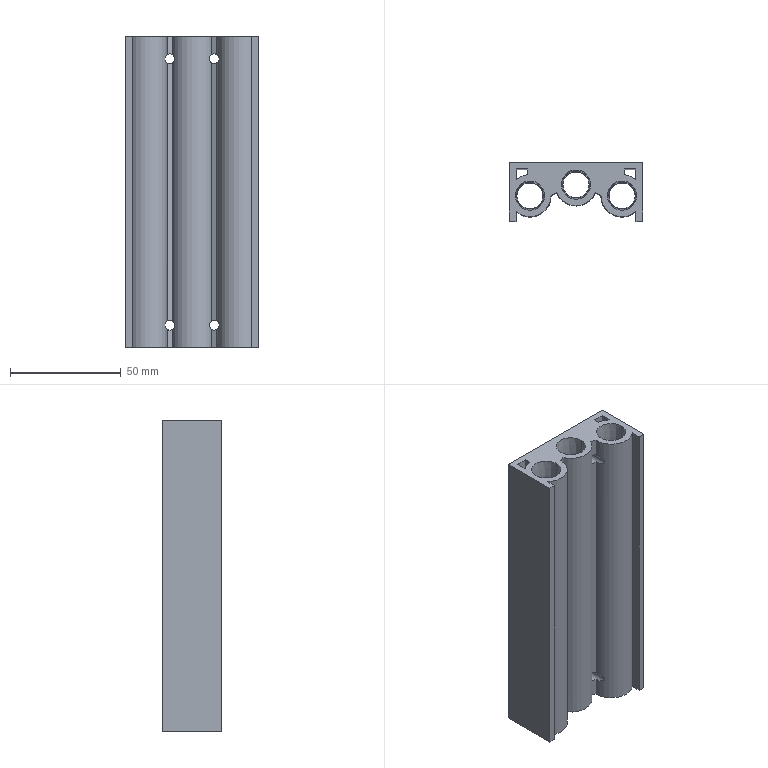Part | SolidWorks | features 3DProfileFeature 3, HoleWzd 3, Cut 1, Extrusion 1, LPattern 1 | 1 solid | 201 faces | box 60 x 26.5 x 140 mm | volume 117754 mm3 | cylinder 92 | cone 82 | plane 27 | commonest cylinder face diameters 6.2 x42 2.5 x28 4.5 x8 19 x8 11.8 x6